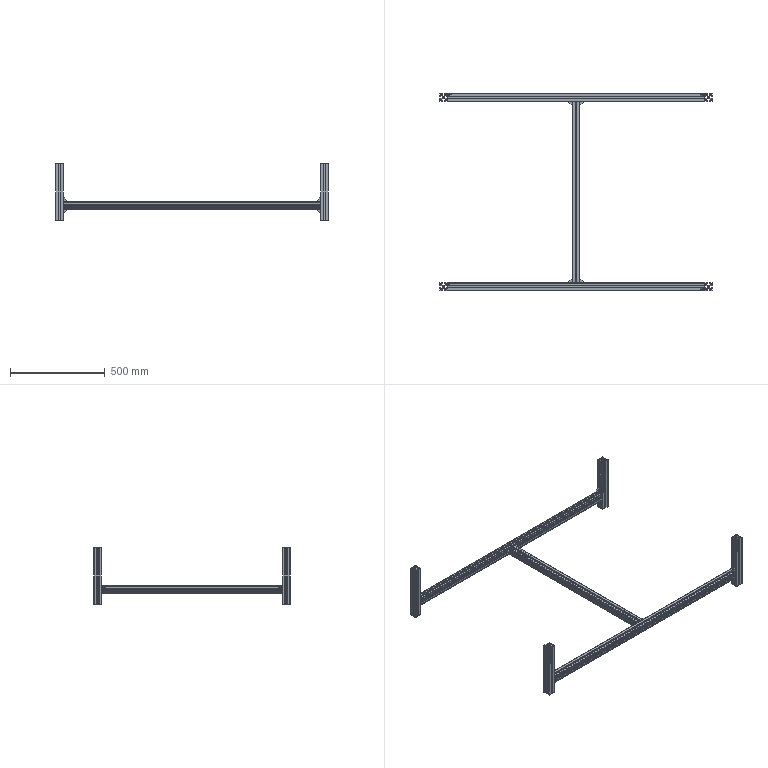Part | SolidWorks | features Gusset 12, 3DProfileFeature 1, WeldMemberFeat 1, WeldmentFeature 1 | 19 solids | 452 faces | box 1440 x 1040 x 300 mm | volume 3739294 mm3 | plane 354 | cylinder 98 | commonest cylinder face diameters 8 x56 1 x28 6.8 x14